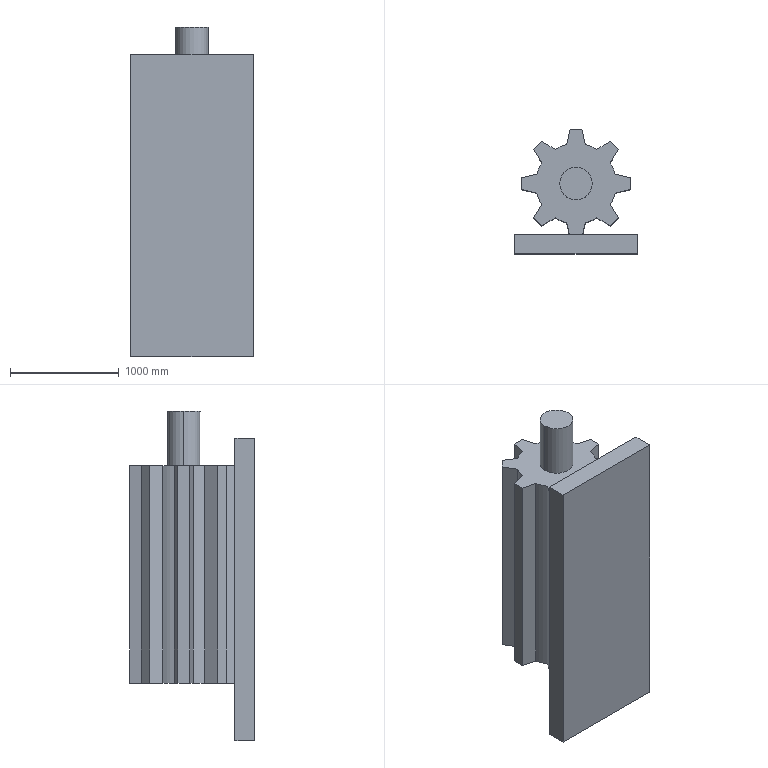Part | SolidWorks | features ICE 5, Extrusion 1 | 1 solid | 42 faces | box 1126 x 1145 x 3030 mm | volume 1733566944 mm3 | plane 32 | cylinder 10 | commonest cylinder face diameters 738.774 x8 300 x2
STEP:
#1=CARTESIAN_POINT('',(150.,0.,-3000.));
#2=VERTEX_POINT('',#1);
#3=CARTESIAN_POINT('',(-150.,0.,-3000.));
#4=VERTEX_POINT('',#3);
#5=CARTESIAN_POINT('',(0.,0.,-3000.));
#6=DIRECTION('',(0.,0.,1.));
#7=DIRECTION('',(-1.,0.,0.));
#8=AXIS2_PLACEMENT_3D('',#5,#6,#7);
#9=CIRCLE('',#8,150.);
#10=EDGE_CURVE('',#2,#4,#9,.T.);
#11=ORIENTED_EDGE('',*,*,#10,.T.);
#12=CARTESIAN_POINT('',(-150.,0.,-2500.));
#13=VERTEX_POINT('',#12);
#14=CARTESIAN_POINT('',(-150.,0.,-3000.));
#15=DIRECTION('',(0.,0.,1.));
#16=VECTOR('',#15,1000.);
#17=LINE('',#14,#16);
#18=EDGE_CURVE('',#4,#13,#17,.T.);
#19=ORIENTED_EDGE('',*,*,#18,.T.);
#20=CARTESIAN_POINT('',(150.,0.,-2500.));
#21=VERTEX_POINT('',#20);
#22=CARTESIAN_POINT('',(0.,0.,-2500.));
#23=DIRECTION('',(0.,0.,-1.));
#24=DIRECTION('',(1.,0.,0.));
#25=AXIS2_PLACEMENT_3D('',#22,#23,#24);
#26=CIRCLE('',#25,150.);
#27=EDGE_CURVE('',#13,#21,#26,.T.);
#28=ORIENTED_EDGE('',*,*,#27,.T.);
#29=CARTESIAN_POINT('',(150.,0.,-3000.));
#30=DIRECTION('',(0.,0.,1.));
#31=VECTOR('',#30,1000.);
#32=LINE('',#29,#31);
#33=EDGE_CURVE('',#2,#21,#32,.T.);
#34=ORIENTED_EDGE('',*,*,#33,.F.);
#35=EDGE_LOOP('',(#11,#19,#28,#34));
#36=FACE_OUTER_BOUND('',#35,.T.);
#37=CARTESIAN_POINT('',(0.,0.,-3000.));
#38=DIRECTION('',(0.,0.,1.));
#39=DIRECTION('',(1.,0.,0.));
#40=AXIS2_PLACEMENT_3D('',#37,#38,#39);
#41=CYLINDRICAL_SURFACE('',#40,150.);
#42=ADVANCED_FACE('',(#36),#41,.T.);
#43=ORIENTED_EDGE('',*,*,#18,.F.);
#44=CARTESIAN_POINT('',(0.,0.,-3000.));
#45=DIRECTION('',(0.,0.,1.));
#46=DIRECTION('',(-1.,0.,0.));
#47=AXIS2_PLACEMENT_3D('',#44,#45,#46);
#48=CIRCLE('',#47,150.);
#49=EDGE_CURVE('',#4,#2,#48,.T.);
#50=ORIENTED_EDGE('',*,*,#49,.T.);
#51=ORIENTED_EDGE('',*,*,#33,.T.);
#52=CARTESIAN_POINT('',(0.,0.,-2500.));
#53=DIRECTION('',(0.,0.,-1.));
#54=DIRECTION('',(1.,0.,0.));
#55=AXIS2_PLACEMENT_3D('',#52,#53,#54);
#56=CIRCLE('',#55,150.);
#57=EDGE_CURVE('',#21,#13,#56,.T.);
#58=ORIENTED_EDGE('',*,*,#57,.T.);
#59=EDGE_LOOP('',(#43,#50,#51,#58));
#60=FACE_OUTER_BOUND('',#59,.T.);
#61=CARTESIAN_POINT('',(0.,0.,-3000.));
#62=DIRECTION('',(0.,0.,1.));
#63=DIRECTION('',(1.,0.,0.));
#64=AXIS2_PLACEMENT_3D('',#61,#62,#63);
#65=CYLINDRICAL_SURFACE('',#64,150.);
#66=ADVANCED_FACE('',(#60),#65,.T.);
#67=CARTESIAN_POINT('',(60.277,-470.229,-5000.));
#68=VERTEX_POINT('',#67);
#69=CARTESIAN_POINT('',(60.277,-470.229,-3000.));
#70=VERTEX_POINT('',#69);
#71=CARTESIAN_POINT('',(60.277,-470.229,-5000.));
#72=DIRECTION('',(0.,0.,1.));
#73=VECTOR('',#72,1000.);
#74=LINE('',#71,#73);
#75=EDGE_CURVE('',#68,#70,#74,.T.);
#76=ORIENTED_EDGE('',*,*,#75,.F.);
#77=CARTESIAN_POINT('',(86.499,-359.116,-5000.));
#78=VERTEX_POINT('',#77);
#79=CARTESIAN_POINT('',(86.499,-359.116,-5000.));
#80=DIRECTION('',(-0.2297,-0.9733,0.));
#81=VECTOR('',#80,1000.);
#82=LINE('',#79,#81);
#83=EDGE_CURVE('',#78,#68,#82,.T.);
#84=ORIENTED_EDGE('',*,*,#83,.F.);
#85=CARTESIAN_POINT('',(86.499,-359.116,-3000.));
#86=VERTEX_POINT('',#85);
#87=CARTESIAN_POINT('',(86.499,-359.116,-5000.));
#88=DIRECTION('',(0.,0.,1.));
#89=VECTOR('',#88,1000.);
#90=LINE('',#87,#89);
#91=EDGE_CURVE('',#78,#86,#90,.T.);
#92=ORIENTED_EDGE('',*,*,#91,.T.);
#93=CARTESIAN_POINT('',(86.499,-359.116,-3000.));
#94=DIRECTION('',(-0.2297,-0.9733,0.));
#95=VECTOR('',#94,1000.);
#96=LINE('',#93,#95);
#97=EDGE_CURVE('',#86,#70,#96,.T.);
#98=ORIENTED_EDGE('',*,*,#97,.T.);
#99=EDGE_LOOP('',(#76,#84,#92,#98));
#100=FACE_OUTER_BOUND('',#99,.T.);
#101=CARTESIAN_POINT('',(86.499,-359.116,-5000.));
#102=DIRECTION('',(-0.9733,0.2297,0.));
#103=DIRECTION('',(-0.2297,-0.9733,0.));
#104=AXIS2_PLACEMENT_3D('',#101,#102,#103);
#105=PLANE('',#104);
#106=ADVANCED_FACE('',(#100),#105,.F.);
#107=CARTESIAN_POINT('',(-60.277,-470.229,-3000.));
#108=VERTEX_POINT('',#107);
#109=CARTESIAN_POINT('',(-60.277,-470.229,-5000.));
#110=VERTEX_POINT('',#109);
#111=CARTESIAN_POINT('',(-60.277,-470.229,-5000.));
#112=DIRECTION('',(0.,0.,-1.));
#113=VECTOR('',#112,1000.);
#114=LINE('',#111,#113);
#115=EDGE_CURVE('',#108,#110,#114,.T.);
#116=ORIENTED_EDGE('',*,*,#115,.F.);
#117=CARTESIAN_POINT('',(-86.499,-359.116,-3000.));
#118=VERTEX_POINT('',#117);
#119=CARTESIAN_POINT('',(-86.499,-359.116,-3000.));
#120=DIRECTION('',(-0.2297,0.9733,0.));
#121=VECTOR('',#120,1000.);
#122=LINE('',#119,#121);
#123=EDGE_CURVE('',#108,#118,#122,.T.);
#124=ORIENTED_EDGE('',*,*,#123,.T.);
#125=CARTESIAN_POINT('',(-86.499,-359.116,-5000.));
#126=VERTEX_POINT('',#125);
#127=CARTESIAN_POINT('',(-86.499,-359.116,-5000.));
#128=DIRECTION('',(0.,0.,1.));
#129=VECTOR('',#128,1000.);
#130=LINE('',#127,#129);
#131=EDGE_CURVE('',#126,#118,#130,.T.);
#132=ORIENTED_EDGE('',*,*,#131,.F.);
#133=CARTESIAN_POINT('',(-86.499,-359.116,-5000.));
#134=DIRECTION('',(-0.2297,0.9733,0.));
#135=VECTOR('',#134,1000.);
#136=LINE('',#133,#135);
#137=EDGE_CURVE('',#110,#126,#136,.T.);
#138=ORIENTED_EDGE('',*,*,#137,.F.);
#139=EDGE_LOOP('',(#116,#124,#132,#138));
#140=FACE_OUTER_BOUND('',#139,.T.);
#141=CARTESIAN_POINT('',(-86.499,-359.116,-5000.));
#142=DIRECTION('',(0.9733,0.2297,0.));
#143=DIRECTION('',(-0.2297,0.9733,0.));
#144=AXIS2_PLACEMENT_3D('',#141,#142,#143);
#145=PLANE('',#144);
#146=ADVANCED_FACE('',(#140),#145,.F.);
#147=ORIENTED_EDGE('',*,*,#83,.T.);
#148=CARTESIAN_POINT('',(0.,-470.229,-5000.));
#149=DIRECTION('',(-1.,0.,0.));
#150=VECTOR('',#149,1000.);
#151=LINE('',#148,#150);
#152=EDGE_CURVE('',#68,#110,#151,.T.);
#153=ORIENTED_EDGE('',*,*,#152,.T.);
#154=ORIENTED_EDGE('',*,*,#137,.T.);
#155=CARTESIAN_POINT('',(-192.769,-315.098,-5000.));
#156=VERTEX_POINT('',#155);
#157=CARTESIAN_POINT('',(0.,0.,-5000.));
#158=DIRECTION('',(0.,0.,-1.));
#159=DIRECTION('',(-1.,0.,0.));
#160=AXIS2_PLACEMENT_3D('',#157,#158,#159);
#161=CIRCLE('',#160,369.387);
#162=EDGE_CURVE('',#126,#156,#161,.T.);
#163=ORIENTED_EDGE('',*,*,#162,.T.);
#164=CARTESIAN_POINT('',(-313.695,-389.845,-5000.));
#165=VERTEX_POINT('',#164);
#166=CARTESIAN_POINT('',(-192.769,-315.098,-5000.));
#167=DIRECTION('',(-0.8506,-0.5258,0.));
#168=VECTOR('',#167,1000.);
#169=LINE('',#166,#168);
#170=EDGE_CURVE('',#156,#165,#169,.T.);
#171=ORIENTED_EDGE('',*,*,#170,.T.);
#172=CARTESIAN_POINT('',(-389.845,-313.695,-5000.));
#173=VERTEX_POINT('',#172);
#174=CARTESIAN_POINT('',(-389.845,-313.695,-5000.));
#175=DIRECTION('',(-0.7071,0.7071,0.));
#176=VECTOR('',#175,1000.);
#177=LINE('',#174,#176);
#178=EDGE_CURVE('',#165,#173,#177,.T.);
#179=ORIENTED_EDGE('',*,*,#178,.T.);
#180=CARTESIAN_POINT('',(-315.098,-192.769,-5000.));
#181=VERTEX_POINT('',#180);
#182=CARTESIAN_POINT('',(-315.098,-192.769,-5000.));
#183=DIRECTION('',(0.5258,0.8506,0.));
#184=VECTOR('',#183,1000.);
#185=LINE('',#182,#184);
#186=EDGE_CURVE('',#173,#181,#185,.T.);
#187=ORIENTED_EDGE('',*,*,#186,.T.);
#188=CARTESIAN_POINT('',(-359.116,-86.499,-5000.));
#189=VERTEX_POINT('',#188);
#190=CARTESIAN_POINT('',(0.,0.,-5000.));
#191=DIRECTION('',(0.,0.,-1.));
#192=DIRECTION('',(-1.,0.,0.));
#193=AXIS2_PLACEMENT_3D('',#190,#191,#192);
#194=CIRCLE('',#193,369.387);
#195=EDGE_CURVE('',#181,#189,#194,.T.);
#196=ORIENTED_EDGE('',*,*,#195,.T.);
#197=CARTESIAN_POINT('',(-497.478,-53.847,-5000.));
#198=VERTEX_POINT('',#197);
#199=CARTESIAN_POINT('',(-359.116,-86.499,-5000.));
#200=DIRECTION('',(-0.9733,0.2297,0.));
#201=VECTOR('',#200,1000.);
#202=LINE('',#199,#201);
#203=EDGE_CURVE('',#189,#198,#202,.T.);
#204=ORIENTED_EDGE('',*,*,#203,.T.);
#205=CARTESIAN_POINT('',(-497.478,53.847,-5000.));
#206=VERTEX_POINT('',#205);
#207=CARTESIAN_POINT('',(-497.478,53.847,-5000.));
#208=DIRECTION('',(0.,1.,0.));
#209=VECTOR('',#208,1000.);
#210=LINE('',#207,#209);
#211=EDGE_CURVE('',#198,#206,#210,.T.);
#212=ORIENTED_EDGE('',*,*,#211,.T.);
#213=CARTESIAN_POINT('',(-359.116,86.499,-5000.));
#214=VERTEX_POINT('',#213);
#215=CARTESIAN_POINT('',(-359.116,86.499,-5000.));
#216=DIRECTION('',(0.9733,0.2297,0.));
#217=VECTOR('',#216,1000.);
#218=LINE('',#215,#217);
#219=EDGE_CURVE('',#206,#214,#218,.T.);
#220=ORIENTED_EDGE('',*,*,#219,.T.);
#221=CARTESIAN_POINT('',(-315.098,192.769,-5000.));
#222=VERTEX_POINT('',#221);
#223=CARTESIAN_POINT('',(0.,0.,-5000.));
#224=DIRECTION('',(0.,0.,-1.));
#225=DIRECTION('',(-1.,0.,0.));
#226=AXIS2_PLACEMENT_3D('',#223,#224,#225);
#227=CIRCLE('',#226,369.387);
#228=EDGE_CURVE('',#214,#222,#227,.T.);
#229=ORIENTED_EDGE('',*,*,#228,.T.);
#230=CARTESIAN_POINT('',(-389.845,313.695,-5000.));
#231=VERTEX_POINT('',#230);
#232=CARTESIAN_POINT('',(-315.098,192.769,-5000.));
#233=DIRECTION('',(-0.5258,0.8506,0.));
#234=VECTOR('',#233,1000.);
#235=LINE('',#232,#234);
#236=EDGE_CURVE('',#222,#231,#235,.T.);
#237=ORIENTED_EDGE('',*,*,#236,.T.);
#238=CARTESIAN_POINT('',(-313.695,389.845,-5000.));
#239=VERTEX_POINT('',#238);
#240=CARTESIAN_POINT('',(-313.695,389.845,-5000.));
#241=DIRECTION('',(0.7071,0.7071,0.));
#242=VECTOR('',#241,1000.);
#243=LINE('',#240,#242);
#244=EDGE_CURVE('',#231,#239,#243,.T.);
#245=ORIENTED_EDGE('',*,*,#244,.T.);
#246=CARTESIAN_POINT('',(-192.769,315.098,-5000.));
#247=VERTEX_POINT('',#246);
#248=CARTESIAN_POINT('',(-192.769,315.098,-5000.));
#249=DIRECTION('',(0.8506,-0.5258,0.));
#250=VECTOR('',#249,1000.);
#251=LINE('',#248,#250);
#252=EDGE_CURVE('',#239,#247,#251,.T.);
#253=ORIENTED_EDGE('',*,*,#252,.T.);
#254=CARTESIAN_POINT('',(-86.499,359.116,-5000.));
#255=VERTEX_POINT('',#254);
#256=CARTESIAN_POINT('',(0.,0.,-5000.));
#257=DIRECTION('',(0.,0.,-1.));
#258=DIRECTION('',(-1.,0.,0.));
#259=AXIS2_PLACEMENT_3D('',#256,#257,#258);
#260=CIRCLE('',#259,369.387);
#261=EDGE_CURVE('',#247,#255,#260,.T.);
#262=ORIENTED_EDGE('',*,*,#261,.T.);
#263=CARTESIAN_POINT('',(-53.847,497.478,-5000.));
#264=VERTEX_POINT('',#263);
#265=CARTESIAN_POINT('',(-86.499,359.116,-5000.));
#266=DIRECTION('',(0.2297,0.9733,0.));
#267=VECTOR('',#266,1000.);
#268=LINE('',#265,#267);
#269=EDGE_CURVE('',#255,#264,#268,.T.);
#270=ORIENTED_EDGE('',*,*,#269,.T.);
#271=CARTESIAN_POINT('',(53.847,497.478,-5000.));
#272=VERTEX_POINT('',#271);
#273=CARTESIAN_POINT('',(53.847,497.478,-5000.));
#274=DIRECTION('',(1.,0.,0.));
#275=VECTOR('',#274,1000.);
#276=LINE('',#273,#275);
#277=EDGE_CURVE('',#264,#272,#276,.T.);
#278=ORIENTED_EDGE('',*,*,#277,.T.);
#279=CARTESIAN_POINT('',(86.499,359.116,-5000.));
#280=VERTEX_POINT('',#279);
#281=CARTESIAN_POINT('',(86.499,359.116,-5000.));
#282=DIRECTION('',(0.2297,-0.9733,0.));
#283=VECTOR('',#282,1000.);
#284=LINE('',#281,#283);
#285=EDGE_CURVE('',#272,#280,#284,.T.);
#286=ORIENTED_EDGE('',*,*,#285,.T.);
#287=CARTESIAN_POINT('',(192.769,315.098,-5000.));
#288=VERTEX_POINT('',#287);
#289=CARTESIAN_POINT('',(0.,0.,-5000.));
#290=DIRECTION('',(0.,0.,-1.));
#291=DIRECTION('',(-1.,0.,0.));
#292=AXIS2_PLACEMENT_3D('',#289,#290,#291);
#293=CIRCLE('',#292,369.387);
#294=EDGE_CURVE('',#280,#288,#293,.T.);
#295=ORIENTED_EDGE('',*,*,#294,.T.);
#296=CARTESIAN_POINT('',(313.695,389.845,-5000.));
#297=VERTEX_POINT('',#296);
#298=CARTESIAN_POINT('',(192.769,315.098,-5000.));
#299=DIRECTION('',(0.8506,0.5258,0.));
#300=VECTOR('',#299,1000.);
#301=LINE('',#298,#300);
#302=EDGE_CURVE('',#288,#297,#301,.T.);
#303=ORIENTED_EDGE('',*,*,#302,.T.);
#304=CARTESIAN_POINT('',(389.845,313.695,-5000.));
#305=VERTEX_POINT('',#304);
#306=CARTESIAN_POINT('',(389.845,313.695,-5000.));
#307=DIRECTION('',(0.7071,-0.7071,0.));
#308=VECTOR('',#307,1000.);
#309=LINE('',#306,#308);
#310=EDGE_CURVE('',#297,#305,#309,.T.);
#311=ORIENTED_EDGE('',*,*,#310,.T.);
#312=CARTESIAN_POINT('',(315.098,192.769,-5000.));
#313=VERTEX_POINT('',#312);
#314=CARTESIAN_POINT('',(315.098,192.769,-5000.));
#315=DIRECTION('',(-0.5258,-0.8506,0.));
#316=VECTOR('',#315,1000.);
#317=LINE('',#314,#316);
#318=EDGE_CURVE('',#305,#313,#317,.T.);
#319=ORIENTED_EDGE('',*,*,#318,.T.);
#320=CARTESIAN_POINT('',(359.116,86.499,-5000.));
#321=VERTEX_POINT('',#320);
#322=CARTESIAN_POINT('',(0.,0.,-5000.));
#323=DIRECTION('',(0.,0.,-1.));
#324=DIRECTION('',(-1.,0.,0.));
#325=AXIS2_PLACEMENT_3D('',#322,#323,#324);
#326=CIRCLE('',#325,369.387);
#327=EDGE_CURVE('',#313,#321,#326,.T.);
#328=ORIENTED_EDGE('',*,*,#327,.T.);
#329=CARTESIAN_POINT('',(497.478,53.847,-5000.));
#330=VERTEX_POINT('',#329);
#331=CARTESIAN_POINT('',(359.116,86.499,-5000.));
#332=DIRECTION('',(0.9733,-0.2297,0.));
#333=VECTOR('',#332,1000.);
#334=LINE('',#331,#333);
#335=EDGE_CURVE('',#321,#330,#334,.T.);
#336=ORIENTED_EDGE('',*,*,#335,.T.);
#337=CARTESIAN_POINT('',(497.478,-53.847,-5000.));
#338=VERTEX_POINT('',#337);
#339=CARTESIAN_POINT('',(497.478,-53.847,-5000.));
#340=DIRECTION('',(0.,-1.,0.));
#341=VECTOR('',#340,1000.);
#342=LINE('',#339,#341);
#343=EDGE_CURVE('',#330,#338,#342,.T.);
#344=ORIENTED_EDGE('',*,*,#343,.T.);
#345=CARTESIAN_POINT('',(359.116,-86.499,-5000.));
#346=VERTEX_POINT('',#345);
#347=CARTESIAN_POINT('',(359.116,-86.499,-5000.));
#348=DIRECTION('',(-0.9733,-0.2297,0.));
#349=VECTOR('',#348,1000.);
#350=LINE('',#347,#349);
#351=EDGE_CURVE('',#338,#346,#350,.T.);
#352=ORIENTED_EDGE('',*,*,#351,.T.);
#353=CARTESIAN_POINT('',(315.098,-192.769,-5000.));
#354=VERTEX_POINT('',#353);
#355=CARTESIAN_POINT('',(0.,0.,-5000.));
#356=DIRECTION('',(0.,0.,-1.));
#357=DIRECTION('',(-1.,0.,0.));
#358=AXIS2_PLACEMENT_3D('',#355,#356,#357);
#359=CIRCLE('',#358,369.387);
#360=EDGE_CURVE('',#346,#354,#359,.T.);
#361=ORIENTED_EDGE('',*,*,#360,.T.);
#362=CARTESIAN_POINT('',(389.845,-313.695,-5000.));
#363=VERTEX_POINT('',#362);
#364=CARTESIAN_POINT('',(315.098,-192.769,-5000.));
#365=DIRECTION('',(0.5258,-0.8506,0.));
#366=VECTOR('',#365,1000.);
#367=LINE('',#364,#366);
#368=EDGE_CURVE('',#354,#363,#367,.T.);
#369=ORIENTED_EDGE('',*,*,#368,.T.);
#370=CARTESIAN_POINT('',(313.695,-389.845,-5000.));
#371=VERTEX_POINT('',#370);
#372=CARTESIAN_POINT('',(313.695,-389.845,-5000.));
#373=DIRECTION('',(-0.7071,-0.7071,0.));
#374=VECTOR('',#373,1000.);
#375=LINE('',#372,#374);
#376=EDGE_CURVE('',#363,#371,#375,.T.);
#377=ORIENTED_EDGE('',*,*,#376,.T.);
#378=CARTESIAN_POINT('',(192.769,-315.098,-5000.));
#379=VERTEX_POINT('',#378);
#380=CARTESIAN_POINT('',(192.769,-315.098,-5000.));
#381=DIRECTION('',(-0.8506,0.5258,0.));
#382=VECTOR('',#381,1000.);
#383=LINE('',#380,#382);
#384=EDGE_CURVE('',#371,#379,#383,.T.);
#385=ORIENTED_EDGE('',*,*,#384,.T.);
#386=CARTESIAN_POINT('',(0.,0.,-5000.));
#387=DIRECTION('',(0.,0.,-1.));
#388=DIRECTION('',(-1.,0.,0.));
#389=AXIS2_PLACEMENT_3D('',#386,#387,#388);
#390=CIRCLE('',#389,369.387);
#391=EDGE_CURVE('',#379,#78,#390,.T.);
#392=ORIENTED_EDGE('',*,*,#391,.T.);
#393=EDGE_LOOP('',(#147,#153,#154,#163,#171,#179,#187,#196,#204,#212,#220,#229,#237,#245,#253,#262,#270,#278,#286,#295,#303,#311,#319,#328,#336,#344,#352,#361,#369,#377,#385,#392));
#394=FACE_OUTER_BOUND('',#393,.T.);
#395=CARTESIAN_POINT('',(0.,0.,-5000.));
#396=DIRECTION('',(0.,0.,-1.));
#397=DIRECTION('',(-1.,0.,0.));
#398=AXIS2_PLACEMENT_3D('',#395,#396,#397);
#399=PLANE('',#398);
#400=ADVANCED_FACE('',(#394),#399,.T.);
#401=ORIENTED_EDGE('',*,*,#10,.F.);
#402=ORIENTED_EDGE('',*,*,#49,.F.);
#403=EDGE_LOOP('',(#401,#402));
#404=FACE_BOUND('',#403,.T.);
#405=CARTESIAN_POINT('',(0.,-470.229,-3000.));
#406=DIRECTION('',(-1.,0.,0.));
#407=VECTOR('',#406,1000.);
#408=LINE('',#405,#407);
#409=EDGE_CURVE('',#70,#108,#408,.T.);
#410=ORIENTED_EDGE('',*,*,#409,.F.);
#411=ORIENTED_EDGE('',*,*,#97,.F.);
#412=CARTESIAN_POINT('',(192.769,-315.098,-3000.));
#413=VERTEX_POINT('',#412);
#414=CARTESIAN_POINT('',(0.,0.,-3000.));
#415=DIRECTION('',(0.,0.,-1.));
#416=DIRECTION('',(-1.,0.,0.));
#417=AXIS2_PLACEMENT_3D('',#414,#415,#416);
#418=CIRCLE('',#417,369.387);
#419=EDGE_CURVE('',#413,#86,#418,.T.);
#420=ORIENTED_EDGE('',*,*,#419,.F.);
#421=CARTESIAN_POINT('',(313.695,-389.845,-3000.));
#422=VERTEX_POINT('',#421);
#423=CARTESIAN_POINT('',(192.769,-315.098,-3000.));
#424=DIRECTION('',(-0.8506,0.5258,0.));
#425=VECTOR('',#424,1000.);
#426=LINE('',#423,#425);
#427=EDGE_CURVE('',#422,#413,#426,.T.);
#428=ORIENTED_EDGE('',*,*,#427,.F.);
#429=CARTESIAN_POINT('',(389.845,-313.695,-3000.));
#430=VERTEX_POINT('',#429);
#431=CARTESIAN_POINT('',(313.695,-389.845,-3000.));
#432=DIRECTION('',(-0.7071,-0.7071,0.));
#433=VECTOR('',#432,1000.);
#434=LINE('',#431,#433);
#435=EDGE_CURVE('',#430,#422,#434,.T.);
#436=ORIENTED_EDGE('',*,*,#435,.F.);
#437=CARTESIAN_POINT('',(315.098,-192.769,-3000.));
#438=VERTEX_POINT('',#437);
#439=CARTESIAN_POINT('',(315.098,-192.769,-3000.));
#440=DIRECTION('',(0.5258,-0.8506,0.));
#441=VECTOR('',#440,1000.);
#442=LINE('',#439,#441);
#443=EDGE_CURVE('',#438,#430,#442,.T.);
#444=ORIENTED_EDGE('',*,*,#443,.F.);
#445=CARTESIAN_POINT('',(359.116,-86.499,-3000.));
#446=VERTEX_POINT('',#445);
#447=CARTESIAN_POINT('',(0.,0.,-3000.));
#448=DIRECTION('',(0.,0.,-1.));
#449=DIRECTION('',(-1.,0.,0.));
#450=AXIS2_PLACEMENT_3D('',#447,#448,#449);
#451=CIRCLE('',#450,369.387);
#452=EDGE_CURVE('',#446,#438,#451,.T.);
#453=ORIENTED_EDGE('',*,*,#452,.F.);
#454=CARTESIAN_POINT('',(497.478,-53.847,-3000.));
#455=VERTEX_POINT('',#454);
#456=CARTESIAN_POINT('',(359.116,-86.499,-3000.));
#457=DIRECTION('',(-0.9733,-0.2297,0.));
#458=VECTOR('',#457,1000.);
#459=LINE('',#456,#458);
#460=EDGE_CURVE('',#455,#446,#459,.T.);
#461=ORIENTED_EDGE('',*,*,#460,.F.);
#462=CARTESIAN_POINT('',(497.478,53.847,-3000.));
#463=VERTEX_POINT('',#462);
#464=CARTESIAN_POINT('',(497.478,-53.847,-3000.));
#465=DIRECTION('',(0.,-1.,0.));
#466=VECTOR('',#465,1000.);
#467=LINE('',#464,#466);
#468=EDGE_CURVE('',#463,#455,#467,.T.);
#469=ORIENTED_EDGE('',*,*,#468,.F.);
#470=CARTESIAN_POINT('',(359.116,86.499,-3000.));
#471=VERTEX_POINT('',#470);
#472=CARTESIAN_POINT('',(359.116,86.499,-3000.));
#473=DIRECTION('',(0.9733,-0.2297,0.));
#474=VECTOR('',#473,1000.);
#475=LINE('',#472,#474);
#476=EDGE_CURVE('',#471,#463,#475,.T.);
#477=ORIENTED_EDGE('',*,*,#476,.F.);
#478=CARTESIAN_POINT('',(315.098,192.769,-3000.));
#479=VERTEX_POINT('',#478);
#480=CARTESIAN_POINT('',(0.,0.,-3000.));
#481=DIRECTION('',(0.,0.,-1.));
#482=DIRECTION('',(-1.,0.,0.));
#483=AXIS2_PLACEMENT_3D('',#480,#481,#482);
#484=CIRCLE('',#483,369.387);
#485=EDGE_CURVE('',#479,#471,#484,.T.);
#486=ORIENTED_EDGE('',*,*,#485,.F.);
#487=CARTESIAN_POINT('',(389.845,313.695,-3000.));
#488=VERTEX_POINT('',#487);
#489=CARTESIAN_POINT('',(315.098,192.769,-3000.));
#490=DIRECTION('',(-0.5258,-0.8506,0.));
#491=VECTOR('',#490,1000.);
#492=LINE('',#489,#491);
#493=EDGE_CURVE('',#488,#479,#492,.T.);
#494=ORIENTED_EDGE('',*,*,#493,.F.);
#495=CARTESIAN_POINT('',(313.695,389.845,-3000.));
#496=VERTEX_POINT('',#495);
#497=CARTESIAN_POINT('',(389.845,313.695,-3000.));
#498=DIRECTION('',(0.7071,-0.7071,0.));
#499=VECTOR('',#498,1000.);
#500=LINE('',#497,#499);
#501=EDGE_CURVE('',#496,#488,#500,.T.);
#502=ORIENTED_EDGE('',*,*,#501,.F.);
#503=CARTESIAN_POINT('',(192.769,315.098,-3000.));
#504=VERTEX_POINT('',#503);
#505=CARTESIAN_POINT('',(192.769,315.098,-3000.));
#506=DIRECTION('',(0.8506,0.5258,0.));
#507=VECTOR('',#506,1000.);
#508=LINE('',#505,#507);
#509=EDGE_CURVE('',#504,#496,#508,.T.);
#510=ORIENTED_EDGE('',*,*,#509,.F.);
#511=CARTESIAN_POINT('',(86.499,359.116,-3000.));
#512=VERTEX_POINT('',#511);
#513=CARTESIAN_POINT('',(0.,0.,-3000.));
#514=DIRECTION('',(0.,0.,-1.));
#515=DIRECTION('',(-1.,0.,0.));
#516=AXIS2_PLACEMENT_3D('',#513,#514,#515);
#517=CIRCLE('',#516,369.387);
#518=EDGE_CURVE('',#512,#504,#517,.T.);
#519=ORIENTED_EDGE('',*,*,#518,.F.);
#520=CARTESIAN_POINT('',(53.847,497.478,-3000.));
#521=VERTEX_POINT('',#520);
#522=CARTESIAN_POINT('',(86.499,359.116,-3000.));
#523=DIRECTION('',(0.2297,-0.9733,0.));
#524=VECTOR('',#523,1000.);
#525=LINE('',#522,#524);
#526=EDGE_CURVE('',#521,#512,#525,.T.);
#527=ORIENTED_EDGE('',*,*,#526,.F.);
#528=CARTESIAN_POINT('',(-53.847,497.478,-3000.));
#529=VERTEX_POINT('',#528);
#530=CARTESIAN_POINT('',(53.847,497.478,-3000.));
#531=DIRECTION('',(1.,0.,0.));
#532=VECTOR('',#531,1000.);
#533=LINE('',#530,#532);
#534=EDGE_CURVE('',#529,#521,#533,.T.);
#535=ORIENTED_EDGE('',*,*,#534,.F.);
#536=CARTESIAN_POINT('',(-86.499,359.116,-3000.));
#537=VERTEX_POINT('',#536);
#538=CARTESIAN_POINT('',(-86.499,359.116,-3000.));
#539=DIRECTION('',(0.2297,0.9733,0.));
#540=VECTOR('',#539,1000.);
#541=LINE('',#538,#540);
#542=EDGE_CURVE('',#537,#529,#541,.T.);
#543=ORIENTED_EDGE('',*,*,#542,.F.);
#544=CARTESIAN_POINT('',(-192.769,315.098,-3000.));
#545=VERTEX_POINT('',#544);
#546=CARTESIAN_POINT('',(0.,0.,-3000.));
#547=DIRECTION('',(0.,0.,-1.));
#548=DIRECTION('',(-1.,0.,0.));
#549=AXIS2_PLACEMENT_3D('',#546,#547,#548);
#550=CIRCLE('',#549,369.387);
#551=EDGE_CURVE('',#545,#537,#550,.T.);
#552=ORIENTED_EDGE('',*,*,#551,.F.);
#553=CARTESIAN_POINT('',(-313.695,389.845,-3000.));
#554=VERTEX_POINT('',#553);
#555=CARTESIAN_POINT('',(-192.769,315.098,-3000.));
#556=DIRECTION('',(0.8506,-0.5258,0.));
#557=VECTOR('',#556,1000.);
#558=LINE('',#555,#557);
#559=EDGE_CURVE('',#554,#545,#558,.T.);
#560=ORIENTED_EDGE('',*,*,#559,.F.);
#561=CARTESIAN_POINT('',(-389.845,313.695,-3000.));
#562=VERTEX_POINT('',#561);
#563=CARTESIAN_POINT('',(-313.695,389.845,-3000.));
#564=DIRECTION('',(0.7071,0.7071,0.));
#565=VECTOR('',#564,1000.);
#566=LINE('',#563,#565);
#567=EDGE_CURVE('',#562,#554,#566,.T.);
#568=ORIENTED_EDGE('',*,*,#567,.F.);
#569=CARTESIAN_POINT('',(-315.098,192.769,-3000.));
#570=VERTEX_POINT('',#569);
#571=CARTESIAN_POINT('',(-315.098,192.769,-3000.));
#572=DIRECTION('',(-0.5258,0.8506,0.));
#573=VECTOR('',#572,1000.);
#574=LINE('',#571,#573);
#575=EDGE_CURVE('',#570,#562,#574,.T.);
#576=ORIENTED_EDGE('',*,*,#575,.F.);
#577=CARTESIAN_POINT('',(-359.116,86.499,-3000.));
#578=VERTEX_POINT('',#577);
#579=CARTESIAN_POINT('',(0.,0.,-3000.));
#580=DIRECTION('',(0.,0.,-1.));
#581=DIRECTION('',(-1.,0.,0.));
#582=AXIS2_PLACEMENT_3D('',#579,#580,#581);
#583=CIRCLE('',#582,369.387);
#584=EDGE_CURVE('',#578,#570,#583,.T.);
#585=ORIENTED_EDGE('',*,*,#584,.F.);
#586=CARTESIAN_POINT('',(-497.478,53.847,-3000.));
#587=VERTEX_POINT('',#586);
#588=CARTESIAN_POINT('',(-359.116,86.499,-3000.));
#589=DIRECTION('',(0.9733,0.2297,0.));
#590=VECTOR('',#589,1000.);
#591=LINE('',#588,#590);
#592=EDGE_CURVE('',#587,#578,#591,.T.);
#593=ORIENTED_EDGE('',*,*,#592,.F.);
#594=CARTESIAN_POINT('',(-497.478,-53.847,-3000.));
#595=VERTEX_POINT('',#594);
#596=CARTESIAN_POINT('',(-497.478,53.847,-3000.));
#597=DIRECTION('',(0.,1.,0.));
#598=VECTOR('',#597,1000.);
#599=LINE('',#596,#598);
#600=EDGE_CURVE('',#595,#587,#599,.T.);
#601=ORIENTED_EDGE('',*,*,#600,.F.);
#602=CARTESIAN_POINT('',(-359.116,-86.499,-3000.));
#603=VERTEX_POINT('',#602);
#604=CARTESIAN_POINT('',(-359.116,-86.499,-3000.));
#605=DIRECTION('',(-0.9733,0.2297,0.));
#606=VECTOR('',#605,1000.);
#607=LINE('',#604,#606);
#608=EDGE_CURVE('',#603,#595,#607,.T.);
#609=ORIENTED_EDGE('',*,*,#608,.F.);
#610=CARTESIAN_POINT('',(-315.098,-192.769,-3000.));
#611=VERTEX_POINT('',#610);
#612=CARTESIAN_POINT('',(0.,0.,-3000.));
#613=DIRECTION('',(0.,0.,-1.));
#614=DIRECTION('',(-1.,0.,0.));
#615=AXIS2_PLACEMENT_3D('',#612,#613,#614);
#616=CIRCLE('',#615,369.387);
#617=EDGE_CURVE('',#611,#603,#616,.T.);
#618=ORIENTED_EDGE('',*,*,#617,.F.);
#619=CARTESIAN_POINT('',(-389.845,-313.695,-3000.));
#620=VERTEX_POINT('',#619);
#621=CARTESIAN_POINT('',(-315.098,-192.769,-3000.));
#622=DIRECTION('',(0.5258,0.8506,0.));
#623=VECTOR('',#622,1000.);
#624=LINE('',#621,#623);
#625=EDGE_CURVE('',#620,#611,#624,.T.);
#626=ORIENTED_EDGE('',*,*,#625,.F.);
#627=CARTESIAN_POINT('',(-313.695,-389.845,-3000.));
#628=VERTEX_POINT('',#627);
#629=CARTESIAN_POINT('',(-389.845,-313.695,-3000.));
#630=DIRECTION('',(-0.7071,0.7071,0.));
#631=VECTOR('',#630,1000.);
#632=LINE('',#629,#631);
#633=EDGE_CURVE('',#628,#620,#632,.T.);
#634=ORIENTED_EDGE('',*,*,#633,.F.);
#635=CARTESIAN_POINT('',(-192.769,-315.098,-3000.));
#636=VERTEX_POINT('',#635);
#637=CARTESIAN_POINT('',(-192.769,-315.098,-3000.));
#638=DIRECTION('',(-0.8506,-0.5258,0.));
#639=VECTOR('',#638,1000.);
#640=LINE('',#637,#639);
#641=EDGE_CURVE('',#636,#628,#640,.T.);
#642=ORIENTED_EDGE('',*,*,#641,.F.);
#643=CARTESIAN_POINT('',(0.,0.,-3000.));
#644=DIRECTION('',(0.,0.,-1.));
#645=DIRECTION('',(-1.,0.,0.));
#646=AXIS2_PLACEMENT_3D('',#643,#644,#645);
#647=CIRCLE('',#646,369.387);
#648=EDGE_CURVE('',#118,#636,#647,.T.);
#649=ORIENTED_EDGE('',*,*,#648,.F.);
#650=ORIENTED_EDGE('',*,*,#123,.F.);
#651=EDGE_LOOP('',(#410,#411,#420,#428,#436,#444,#453,#461,#469,#477,#486,#494,#502,#510,#519,#527,#535,#543,#552,#560,#568,#576,#585,#593,#601,#609,#618,#626,#634,#642,#649,#650));
#652=FACE_OUTER_BOUND('',#651,.T.);
#653=CARTESIAN_POINT('',(0.,0.,-3000.));
#654=DIRECTION('',(0.,0.,-1.));
#655=DIRECTION('',(-1.,0.,0.));
#656=AXIS2_PLACEMENT_3D('',#653,#654,#655);
#657=PLANE('',#656);
#658=ADVANCED_FACE('',(#404,#652),#657,.F.);
#659=ORIENTED_EDGE('',*,*,#518,.T.);
#660=CARTESIAN_POINT('',(192.769,315.098,-5000.));
#661=DIRECTION('',(0.,0.,1.));
#662=VECTOR('',#661,1000.);
#663=LINE('',#660,#662);
#664=EDGE_CURVE('',#288,#504,#663,.T.);
#665=ORIENTED_EDGE('',*,*,#664,.F.);
#666=ORIENTED_EDGE('',*,*,#294,.F.);
#667=CARTESIAN_POINT('',(86.499,359.116,-5000.));
#668=DIRECTION('',(0.,0.,1.));
#669=VECTOR('',#668,1000.);
#670=LINE('',#667,#669);
#671=EDGE_CURVE('',#280,#512,#670,.T.);
#672=ORIENTED_EDGE('',*,*,#671,.T.);
#673=EDGE_LOOP('',(#659,#665,#666,#672));
#674=FACE_OUTER_BOUND('',#673,.T.);
#675=CARTESIAN_POINT('',(0.,0.,-5000.));
#676=DIRECTION('',(0.,0.,1.));
#677=DIRECTION('',(1.,0.,0.));
#678=AXIS2_PLACEMENT_3D('',#675,#676,#677);
#679=CYLINDRICAL_SURFACE('',#678,369.387);
#680=ADVANCED_FACE('',(#674),#679,.T.);
#681=ORIENTED_EDGE('',*,*,#509,.T.);
#682=CARTESIAN_POINT('',(313.695,389.845,-5000.));
#683=DIRECTION('',(0.,0.,1.));
#684=VECTOR('',#683,1000.);
#685=LINE('',#682,#684);
#686=EDGE_CURVE('',#297,#496,#685,.T.);
#687=ORIENTED_EDGE('',*,*,#686,.F.);
#688=ORIENTED_EDGE('',*,*,#302,.F.);
#689=ORIENTED_EDGE('',*,*,#664,.T.);
#690=EDGE_LOOP('',(#681,#687,#688,#689));
#691=FACE_OUTER_BOUND('',#690,.T.);
#692=CARTESIAN_POINT('',(192.769,315.098,-5000.));
#693=DIRECTION('',(0.5258,-0.8506,0.));
#694=DIRECTION('',(0.8506,0.5258,0.));
#695=AXIS2_PLACEMENT_3D('',#692,#693,#694);
#696=PLANE('',#695);
#697=ADVANCED_FACE('',(#691),#696,.F.);
#698=ORIENTED_EDGE('',*,*,#501,.T.);
#699=CARTESIAN_POINT('',(389.845,313.695,-5000.));
#700=DIRECTION('',(0.,0.,1.));
#701=VECTOR('',#700,1000.);
#702=LINE('',#699,#701);
#703=EDGE_CURVE('',#305,#488,#702,.T.);
#704=ORIENTED_EDGE('',*,*,#703,.F.);
#705=ORIENTED_EDGE('',*,*,#310,.F.);
#706=ORIENTED_EDGE('',*,*,#686,.T.);
#707=EDGE_LOOP('',(#698,#704,#705,#706));
#708=FACE_OUTER_BOUND('',#707,.T.);
#709=CARTESIAN_POINT('',(389.845,313.695,-5000.));
#710=DIRECTION('',(-0.7071,-0.7071,0.));
#711=DIRECTION('',(0.7071,-0.7071,0.));
#712=AXIS2_PLACEMENT_3D('',#709,#710,#711);
#713=PLANE('',#712);
#714=ADVANCED_FACE('',(#708),#713,.F.);
#715=ORIENTED_EDGE('',*,*,#493,.T.);
#716=CARTESIAN_POINT('',(315.098,192.769,-5000.));
#717=DIRECTION('',(0.,0.,1.));
#718=VECTOR('',#717,1000.);
#719=LINE('',#716,#718);
#720=EDGE_CURVE('',#313,#479,#719,.T.);
#721=ORIENTED_EDGE('',*,*,#720,.F.);
#722=ORIENTED_EDGE('',*,*,#318,.F.);
#723=ORIENTED_EDGE('',*,*,#703,.T.);
#724=EDGE_LOOP('',(#715,#721,#722,#723));
#725=FACE_OUTER_BOUND('',#724,.T.);
#726=CARTESIAN_POINT('',(315.098,192.769,-5000.));
#727=DIRECTION('',(-0.8506,0.5258,0.));
#728=DIRECTION('',(-0.5258,-0.8506,0.));
#729=AXIS2_PLACEMENT_3D('',#726,#727,#728);
#730=PLANE('',#729);
#731=ADVANCED_FACE('',(#725),#730,.F.);
#732=ORIENTED_EDGE('',*,*,#485,.T.);
#733=CARTESIAN_POINT('',(359.116,86.499,-5000.));
#734=DIRECTION('',(0.,0.,1.));
#735=VECTOR('',#734,1000.);
#736=LINE('',#733,#735);
#737=EDGE_CURVE('',#321,#471,#736,.T.);
#738=ORIENTED_EDGE('',*,*,#737,.F.);
#739=ORIENTED_EDGE('',*,*,#327,.F.);
#740=ORIENTED_EDGE('',*,*,#720,.T.);
#741=EDGE_LOOP('',(#732,#738,#739,#740));
#742=FACE_OUTER_BOUND('',#741,.T.);
#743=CARTESIAN_POINT('',(0.,0.,-5000.));
#744=DIRECTION('',(0.,0.,1.));
#745=DIRECTION('',(1.,0.,0.));
#746=AXIS2_PLACEMENT_3D('',#743,#744,#745);
#747=CYLINDRICAL_SURFACE('',#746,369.387);
#748=ADVANCED_FACE('',(#742),#747,.T.);
#749=ORIENTED_EDGE('',*,*,#476,.T.);
#750=CARTESIAN_POINT('',(497.478,53.847,-5000.));
#751=DIRECTION('',(0.,0.,1.));
#752=VECTOR('',#751,1000.);
#753=LINE('',#750,#752);
#754=EDGE_CURVE('',#330,#463,#753,.T.);
#755=ORIENTED_EDGE('',*,*,#754,.F.);
#756=ORIENTED_EDGE('',*,*,#335,.F.);
#757=ORIENTED_EDGE('',*,*,#737,.T.);
#758=EDGE_LOOP('',(#749,#755,#756,#757));
#759=FACE_OUTER_BOUND('',#758,.T.);
#760=CARTESIAN_POINT('',(359.116,86.499,-5000.));
#761=DIRECTION('',(-0.2297,-0.9733,0.));
#762=DIRECTION('',(0.9733,-0.2297,0.));
#763=AXIS2_PLACEMENT_3D('',#760,#761,#762);
#764=PLANE('',#763);
#765=ADVANCED_FACE('',(#759),#764,.F.);
#766=ORIENTED_EDGE('',*,*,#468,.T.);
#767=CARTESIAN_POINT('',(497.478,-53.847,-5000.));
#768=DIRECTION('',(0.,0.,1.));
#769=VECTOR('',#768,1000.);
#770=LINE('',#767,#769);
#771=EDGE_CURVE('',#338,#455,#770,.T.);
#772=ORIENTED_EDGE('',*,*,#771,.F.);
#773=ORIENTED_EDGE('',*,*,#343,.F.);
#774=ORIENTED_EDGE('',*,*,#754,.T.);
#775=EDGE_LOOP('',(#766,#772,#773,#774));
#776=FACE_OUTER_BOUND('',#775,.T.);
#777=CARTESIAN_POINT('',(497.478,-53.847,-5000.));
#778=DIRECTION('',(-1.,0.,0.));
#779=DIRECTION('',(0.,0.,1.));
#780=AXIS2_PLACEMENT_3D('',#777,#778,#779);
#781=PLANE('',#780);
#782=ADVANCED_FACE('',(#776),#781,.F.);
#783=ORIENTED_EDGE('',*,*,#460,.T.);
#784=CARTESIAN_POINT('',(359.116,-86.499,-5000.));
#785=DIRECTION('',(0.,0.,1.));
#786=VECTOR('',#785,1000.);
#787=LINE('',#784,#786);
#788=EDGE_CURVE('',#346,#446,#787,.T.);
#789=ORIENTED_EDGE('',*,*,#788,.F.);
#790=ORIENTED_EDGE('',*,*,#351,.F.);
#791=ORIENTED_EDGE('',*,*,#771,.T.);
#792=EDGE_LOOP('',(#783,#789,#790,#791));
#793=FACE_OUTER_BOUND('',#792,.T.);
#794=CARTESIAN_POINT('',(359.116,-86.499,-5000.));
#795=DIRECTION('',(-0.2297,0.9733,0.));
#796=DIRECTION('',(-0.9733,-0.2297,0.));
#797=AXIS2_PLACEMENT_3D('',#794,#795,#796);
#798=PLANE('',#797);
#799=ADVANCED_FACE('',(#793),#798,.F.);
#800=ORIENTED_EDGE('',*,*,#452,.T.);
#801=CARTESIAN_POINT('',(315.098,-192.769,-5000.));
#802=DIRECTION('',(0.,0.,1.));
#803=VECTOR('',#802,1000.);
#804=LINE('',#801,#803);
#805=EDGE_CURVE('',#354,#438,#804,.T.);
#806=ORIENTED_EDGE('',*,*,#805,.F.);
#807=ORIENTED_EDGE('',*,*,#360,.F.);
#808=ORIENTED_EDGE('',*,*,#788,.T.);
#809=EDGE_LOOP('',(#800,#806,#807,#808));
#810=FACE_OUTER_BOUND('',#809,.T.);
#811=CARTESIAN_POINT('',(0.,0.,-5000.));
#812=DIRECTION('',(0.,0.,1.));
#813=DIRECTION('',(1.,0.,0.));
#814=AXIS2_PLACEMENT_3D('',#811,#812,#813);
#815=CYLINDRICAL_SURFACE('',#814,369.387);
#816=ADVANCED_FACE('',(#810),#815,.T.);
#817=ORIENTED_EDGE('',*,*,#443,.T.);
#818=CARTESIAN_POINT('',(389.845,-313.695,-5000.));
#819=DIRECTION('',(0.,0.,1.));
#820=VECTOR('',#819,1000.);
#821=LINE('',#818,#820);
#822=EDGE_CURVE('',#363,#430,#821,.T.);
#823=ORIENTED_EDGE('',*,*,#822,.F.);
#824=ORIENTED_EDGE('',*,*,#368,.F.);
#825=ORIENTED_EDGE('',*,*,#805,.T.);
#826=EDGE_LOOP('',(#817,#823,#824,#825));
#827=FACE_OUTER_BOUND('',#826,.T.);
#828=CARTESIAN_POINT('',(315.098,-192.769,-5000.));
#829=DIRECTION('',(-0.8506,-0.5258,0.));
#830=DIRECTION('',(0.5258,-0.8506,0.));
#831=AXIS2_PLACEMENT_3D('',#828,#829,#830);
#832=PLANE('',#831);
#833=ADVANCED_FACE('',(#827),#832,.F.);
#834=ORIENTED_EDGE('',*,*,#435,.T.);
#835=CARTESIAN_POINT('',(313.695,-389.845,-5000.));
#836=DIRECTION('',(0.,0.,1.));
#837=VECTOR('',#836,1000.);
#838=LINE('',#835,#837);
#839=EDGE_CURVE('',#371,#422,#838,.T.);
#840=ORIENTED_EDGE('',*,*,#839,.F.);
#841=ORIENTED_EDGE('',*,*,#376,.F.);
#842=ORIENTED_EDGE('',*,*,#822,.T.);
#843=EDGE_LOOP('',(#834,#840,#841,#842));
#844=FACE_OUTER_BOUND('',#843,.T.);
#845=CARTESIAN_POINT('',(313.695,-389.845,-5000.));
#846=DIRECTION('',(-0.7071,0.7071,0.));
#847=DIRECTION('',(-0.7071,-0.7071,0.));
#848=AXIS2_PLACEMENT_3D('',#845,#846,#847);
#849=PLANE('',#848);
#850=ADVANCED_FACE('',(#844),#849,.F.);
#851=ORIENTED_EDGE('',*,*,#427,.T.);
#852=CARTESIAN_POINT('',(192.769,-315.098,-5000.));
#853=DIRECTION('',(0.,0.,1.));
#854=VECTOR('',#853,1000.);
#855=LINE('',#852,#854);
#856=EDGE_CURVE('',#379,#413,#855,.T.);
#857=ORIENTED_EDGE('',*,*,#856,.F.);
#858=ORIENTED_EDGE('',*,*,#384,.F.);
#859=ORIENTED_EDGE('',*,*,#839,.T.);
#860=EDGE_LOOP('',(#851,#857,#858,#859));
#861=FACE_OUTER_BOUND('',#860,.T.);
#862=CARTESIAN_POINT('',(192.769,-315.098,-5000.));
#863=DIRECTION('',(0.5258,0.8506,0.));
#864=DIRECTION('',(-0.8506,0.5258,0.));
#865=AXIS2_PLACEMENT_3D('',#862,#863,#864);
#866=PLANE('',#865);
#867=ADVANCED_FACE('',(#861),#866,.F.);
#868=ORIENTED_EDGE('',*,*,#419,.T.);
#869=ORIENTED_EDGE('',*,*,#91,.F.);
#870=ORIENTED_EDGE('',*,*,#391,.F.);
#871=ORIENTED_EDGE('',*,*,#856,.T.);
#872=EDGE_LOOP('',(#868,#869,#870,#871));
#873=FACE_OUTER_BOUND('',#872,.T.);
#874=CARTESIAN_POINT('',(0.,0.,-5000.));
#875=DIRECTION('',(0.,0.,1.));
#876=DIRECTION('',(1.,0.,0.));
#877=AXIS2_PLACEMENT_3D('',#874,#875,#876);
#878=CYLINDRICAL_SURFACE('',#877,369.387);
#879=ADVANCED_FACE('',(#873),#878,.T.);
#880=ORIENTED_EDGE('',*,*,#648,.T.);
#881=CARTESIAN_POINT('',(-192.769,-315.098,-5000.));
#882=DIRECTION('',(0.,0.,1.));
#883=VECTOR('',#882,1000.);
#884=LINE('',#881,#883);
#885=EDGE_CURVE('',#156,#636,#884,.T.);
#886=ORIENTED_EDGE('',*,*,#885,.F.);
#887=ORIENTED_EDGE('',*,*,#162,.F.);
#888=ORIENTED_EDGE('',*,*,#131,.T.);
#889=EDGE_LOOP('',(#880,#886,#887,#888));
#890=FACE_OUTER_BOUND('',#889,.T.);
#891=CARTESIAN_POINT('',(0.,0.,-5000.));
#892=DIRECTION('',(0.,0.,1.));
#893=DIRECTION('',(1.,0.,0.));
#894=AXIS2_PLACEMENT_3D('',#891,#892,#893);
#895=CYLINDRICAL_SURFACE('',#894,369.387);
#896=ADVANCED_FACE('',(#890),#895,.T.);
#897=ORIENTED_EDGE('',*,*,#641,.T.);
#898=CARTESIAN_POINT('',(-313.695,-389.845,-5000.));
#899=DIRECTION('',(0.,0.,1.));
#900=VECTOR('',#899,1000.);
#901=LINE('',#898,#900);
#902=EDGE_CURVE('',#165,#628,#901,.T.);
#903=ORIENTED_EDGE('',*,*,#902,.F.);
#904=ORIENTED_EDGE('',*,*,#170,.F.);
#905=ORIENTED_EDGE('',*,*,#885,.T.);
#906=EDGE_LOOP('',(#897,#903,#904,#905));
#907=FACE_OUTER_BOUND('',#906,.T.);
#908=CARTESIAN_POINT('',(-192.769,-315.098,-5000.));
#909=DIRECTION('',(-0.5258,0.8506,0.));
#910=DIRECTION('',(-0.8506,-0.5258,0.));
#911=AXIS2_PLACEMENT_3D('',#908,#909,#910);
#912=PLANE('',#911);
#913=ADVANCED_FACE('',(#907),#912,.F.);
#914=ORIENTED_EDGE('',*,*,#633,.T.);
#915=CARTESIAN_POINT('',(-389.845,-313.695,-5000.));
#916=DIRECTION('',(0.,0.,1.));
#917=VECTOR('',#916,1000.);
#918=LINE('',#915,#917);
#919=EDGE_CURVE('',#173,#620,#918,.T.);
#920=ORIENTED_EDGE('',*,*,#919,.F.);
#921=ORIENTED_EDGE('',*,*,#178,.F.);
#922=ORIENTED_EDGE('',*,*,#902,.T.);
#923=EDGE_LOOP('',(#914,#920,#921,#922));
#924=FACE_OUTER_BOUND('',#923,.T.);
#925=CARTESIAN_POINT('',(-389.845,-313.695,-5000.));
#926=DIRECTION('',(0.7071,0.7071,0.));
#927=DIRECTION('',(-0.7071,0.7071,0.));
#928=AXIS2_PLACEMENT_3D('',#925,#926,#927);
#929=PLANE('',#928);
#930=ADVANCED_FACE('',(#924),#929,.F.);
#931=ORIENTED_EDGE('',*,*,#625,.T.);
#932=CARTESIAN_POINT('',(-315.098,-192.769,-5000.));
#933=DIRECTION('',(0.,0.,1.));
#934=VECTOR('',#933,1000.);
#935=LINE('',#932,#934);
#936=EDGE_CURVE('',#181,#611,#935,.T.);
#937=ORIENTED_EDGE('',*,*,#936,.F.);
#938=ORIENTED_EDGE('',*,*,#186,.F.);
#939=ORIENTED_EDGE('',*,*,#919,.T.);
#940=EDGE_LOOP('',(#931,#937,#938,#939));
#941=FACE_OUTER_BOUND('',#940,.T.);
#942=CARTESIAN_POINT('',(-315.098,-192.769,-5000.));
#943=DIRECTION('',(0.8506,-0.5258,0.));
#944=DIRECTION('',(0.5258,0.8506,0.));
#945=AXIS2_PLACEMENT_3D('',#942,#943,#944);
#946=PLANE('',#945);
#947=ADVANCED_FACE('',(#941),#946,.F.);
#948=ORIENTED_EDGE('',*,*,#617,.T.);
#949=CARTESIAN_POINT('',(-359.116,-86.499,-5000.));
#950=DIRECTION('',(0.,0.,1.));
#951=VECTOR('',#950,1000.);
#952=LINE('',#949,#951);
#953=EDGE_CURVE('',#189,#603,#952,.T.);
#954=ORIENTED_EDGE('',*,*,#953,.F.);
#955=ORIENTED_EDGE('',*,*,#195,.F.);
#956=ORIENTED_EDGE('',*,*,#936,.T.);
#957=EDGE_LOOP('',(#948,#954,#955,#956));
#958=FACE_OUTER_BOUND('',#957,.T.);
#959=CARTESIAN_POINT('',(0.,0.,-5000.));
#960=DIRECTION('',(0.,0.,1.));
#961=DIRECTION('',(1.,0.,0.));
#962=AXIS2_PLACEMENT_3D('',#959,#960,#961);
#963=CYLINDRICAL_SURFACE('',#962,369.387);
#964=ADVANCED_FACE('',(#958),#963,.T.);
#965=ORIENTED_EDGE('',*,*,#608,.T.);
#966=CARTESIAN_POINT('',(-497.478,-53.847,-5000.));
#967=DIRECTION('',(0.,0.,1.));
#968=VECTOR('',#967,1000.);
#969=LINE('',#966,#968);
#970=EDGE_CURVE('',#198,#595,#969,.T.);
#971=ORIENTED_EDGE('',*,*,#970,.F.);
#972=ORIENTED_EDGE('',*,*,#203,.F.);
#973=ORIENTED_EDGE('',*,*,#953,.T.);
#974=EDGE_LOOP('',(#965,#971,#972,#973));
#975=FACE_OUTER_BOUND('',#974,.T.);
#976=CARTESIAN_POINT('',(-359.116,-86.499,-5000.));
#977=DIRECTION('',(0.2297,0.9733,0.));
#978=DIRECTION('',(-0.9733,0.2297,0.));
#979=AXIS2_PLACEMENT_3D('',#976,#977,#978);
#980=PLANE('',#979);
#981=ADVANCED_FACE('',(#975),#980,.F.);
#982=ORIENTED_EDGE('',*,*,#600,.T.);
#983=CARTESIAN_POINT('',(-497.478,53.847,-5000.));
#984=DIRECTION('',(0.,0.,1.));
#985=VECTOR('',#984,1000.);
#986=LINE('',#983,#985);
#987=EDGE_CURVE('',#206,#587,#986,.T.);
#988=ORIENTED_EDGE('',*,*,#987,.F.);
#989=ORIENTED_EDGE('',*,*,#211,.F.);
#990=ORIENTED_EDGE('',*,*,#970,.T.);
#991=EDGE_LOOP('',(#982,#988,#989,#990));
#992=FACE_OUTER_BOUND('',#991,.T.);
#993=CARTESIAN_POINT('',(-497.478,53.847,-5000.));
#994=DIRECTION('',(1.,0.,0.));
#995=DIRECTION('',(0.,1.,0.));
#996=AXIS2_PLACEMENT_3D('',#993,#994,#995);
#997=PLANE('',#996);
#998=ADVANCED_FACE('',(#992),#997,.F.);
#999=ORIENTED_EDGE('',*,*,#592,.T.);
#1000=CARTESIAN_POINT('',(-359.116,86.499,-5000.));
#1001=DIRECTION('',(0.,0.,1.));
#1002=VECTOR('',#1001,1000.);
#1003=LINE('',#1000,#1002);
#1004=EDGE_CURVE('',#214,#578,#1003,.T.);
#1005=ORIENTED_EDGE('',*,*,#1004,.F.);
#1006=ORIENTED_EDGE('',*,*,#219,.F.);
#1007=ORIENTED_EDGE('',*,*,#987,.T.);
#1008=EDGE_LOOP('',(#999,#1005,#1006,#1007));
#1009=FACE_OUTER_BOUND('',#1008,.T.);
#1010=CARTESIAN_POINT('',(-359.116,86.499,-5000.));
#1011=DIRECTION('',(0.2297,-0.9733,0.));
#1012=DIRECTION('',(0.9733,0.2297,0.));
#1013=AXIS2_PLACEMENT_3D('',#1010,#1011,#1012);
#1014=PLANE('',#1013);
#1015=ADVANCED_FACE('',(#1009),#1014,.F.);
#1016=ORIENTED_EDGE('',*,*,#584,.T.);
#1017=CARTESIAN_POINT('',(-315.098,192.769,-5000.));
#1018=DIRECTION('',(0.,0.,1.));
#1019=VECTOR('',#1018,1000.);
#1020=LINE('',#1017,#1019);
#1021=EDGE_CURVE('',#222,#570,#1020,.T.);
#1022=ORIENTED_EDGE('',*,*,#1021,.F.);
#1023=ORIENTED_EDGE('',*,*,#228,.F.);
#1024=ORIENTED_EDGE('',*,*,#1004,.T.);
#1025=EDGE_LOOP('',(#1016,#1022,#1023,#1024));
#1026=FACE_OUTER_BOUND('',#1025,.T.);
#1027=CARTESIAN_POINT('',(0.,0.,-5000.));
#1028=DIRECTION('',(0.,0.,1.));
#1029=DIRECTION('',(1.,0.,0.));
#1030=AXIS2_PLACEMENT_3D('',#1027,#1028,#1029);
#1031=CYLINDRICAL_SURFACE('',#1030,369.387);
#1032=ADVANCED_FACE('',(#1026),#1031,.T.);
#1033=ORIENTED_EDGE('',*,*,#575,.T.);
#1034=CARTESIAN_POINT('',(-389.845,313.695,-5000.));
#1035=DIRECTION('',(0.,0.,1.));
#1036=VECTOR('',#1035,1000.);
#1037=LINE('',#1034,#1036);
#1038=EDGE_CURVE('',#231,#562,#1037,.T.);
#1039=ORIENTED_EDGE('',*,*,#1038,.F.);
#1040=ORIENTED_EDGE('',*,*,#236,.F.);
#1041=ORIENTED_EDGE('',*,*,#1021,.T.);
#1042=EDGE_LOOP('',(#1033,#1039,#1040,#1041));
#1043=FACE_OUTER_BOUND('',#1042,.T.);
#1044=CARTESIAN_POINT('',(-315.098,192.769,-5000.));
#1045=DIRECTION('',(0.8506,0.5258,0.));
#1046=DIRECTION('',(-0.5258,0.8506,0.));
#1047=AXIS2_PLACEMENT_3D('',#1044,#1045,#1046);
#1048=PLANE('',#1047);
#1049=ADVANCED_FACE('',(#1043),#1048,.F.);
#1050=ORIENTED_EDGE('',*,*,#567,.T.);
#1051=CARTESIAN_POINT('',(-313.695,389.845,-5000.));
#1052=DIRECTION('',(0.,0.,1.));
#1053=VECTOR('',#1052,1000.);
#1054=LINE('',#1051,#1053);
#1055=EDGE_CURVE('',#239,#554,#1054,.T.);
#1056=ORIENTED_EDGE('',*,*,#1055,.F.);
#1057=ORIENTED_EDGE('',*,*,#244,.F.);
#1058=ORIENTED_EDGE('',*,*,#1038,.T.);
#1059=EDGE_LOOP('',(#1050,#1056,#1057,#1058));
#1060=FACE_OUTER_BOUND('',#1059,.T.);
#1061=CARTESIAN_POINT('',(-313.695,389.845,-5000.));
#1062=DIRECTION('',(0.7071,-0.7071,0.));
#1063=DIRECTION('',(0.7071,0.7071,0.));
#1064=AXIS2_PLACEMENT_3D('',#1061,#1062,#1063);
#1065=PLANE('',#1064);
#1066=ADVANCED_FACE('',(#1060),#1065,.F.);
#1067=ORIENTED_EDGE('',*,*,#559,.T.);
#1068=CARTESIAN_POINT('',(-192.769,315.098,-5000.));
#1069=DIRECTION('',(0.,0.,1.));
#1070=VECTOR('',#1069,1000.);
#1071=LINE('',#1068,#1070);
#1072=EDGE_CURVE('',#247,#545,#1071,.T.);
#1073=ORIENTED_EDGE('',*,*,#1072,.F.);
#1074=ORIENTED_EDGE('',*,*,#252,.F.);
#1075=ORIENTED_EDGE('',*,*,#1055,.T.);
#1076=EDGE_LOOP('',(#1067,#1073,#1074,#1075));
#1077=FACE_OUTER_BOUND('',#1076,.T.);
#1078=CARTESIAN_POINT('',(-192.769,315.098,-5000.));
#1079=DIRECTION('',(-0.5258,-0.8506,0.));
#1080=DIRECTION('',(0.8506,-0.5258,0.));
#1081=AXIS2_PLACEMENT_3D('',#1078,#1079,#1080);
#1082=PLANE('',#1081);
#1083=ADVANCED_FACE('',(#1077),#1082,.F.);
#1084=ORIENTED_EDGE('',*,*,#551,.T.);
#1085=CARTESIAN_POINT('',(-86.499,359.116,-5000.));
#1086=DIRECTION('',(0.,0.,1.));
#1087=VECTOR('',#1086,1000.);
#1088=LINE('',#1085,#1087);
#1089=EDGE_CURVE('',#255,#537,#1088,.T.);
#1090=ORIENTED_EDGE('',*,*,#1089,.F.);
#1091=ORIENTED_EDGE('',*,*,#261,.F.);
#1092=ORIENTED_EDGE('',*,*,#1072,.T.);
#1093=EDGE_LOOP('',(#1084,#1090,#1091,#1092));
#1094=FACE_OUTER_BOUND('',#1093,.T.);
#1095=CARTESIAN_POINT('',(0.,0.,-5000.));
#1096=DIRECTION('',(0.,0.,1.));
#1097=DIRECTION('',(1.,0.,0.));
#1098=AXIS2_PLACEMENT_3D('',#1095,#1096,#1097);
#1099=CYLINDRICAL_SURFACE('',#1098,369.387);
#1100=ADVANCED_FACE('',(#1094),#1099,.T.);
#1101=ORIENTED_EDGE('',*,*,#542,.T.);
#1102=CARTESIAN_POINT('',(-53.847,497.478,-5000.));
#1103=DIRECTION('',(0.,0.,1.));
#1104=VECTOR('',#1103,1000.);
#1105=LINE('',#1102,#1104);
#1106=EDGE_CURVE('',#264,#529,#1105,.T.);
#1107=ORIENTED_EDGE('',*,*,#1106,.F.);
#1108=ORIENTED_EDGE('',*,*,#269,.F.);
#1109=ORIENTED_EDGE('',*,*,#1089,.T.);
#1110=EDGE_LOOP('',(#1101,#1107,#1108,#1109));
#1111=FACE_OUTER_BOUND('',#1110,.T.);
#1112=CARTESIAN_POINT('',(-86.499,359.116,-5000.));
#1113=DIRECTION('',(0.9733,-0.2297,0.));
#1114=DIRECTION('',(0.2297,0.9733,0.));
#1115=AXIS2_PLACEMENT_3D('',#1112,#1113,#1114);
#1116=PLANE('',#1115);
#1117=ADVANCED_FACE('',(#1111),#1116,.F.);
#1118=ORIENTED_EDGE('',*,*,#534,.T.);
#1119=CARTESIAN_POINT('',(53.847,497.478,-5000.));
#1120=DIRECTION('',(0.,0.,1.));
#1121=VECTOR('',#1120,1000.);
#1122=LINE('',#1119,#1121);
#1123=EDGE_CURVE('',#272,#521,#1122,.T.);
#1124=ORIENTED_EDGE('',*,*,#1123,.F.);
#1125=ORIENTED_EDGE('',*,*,#277,.F.);
#1126=ORIENTED_EDGE('',*,*,#1106,.T.);
#1127=EDGE_LOOP('',(#1118,#1124,#1125,#1126));
#1128=FACE_OUTER_BOUND('',#1127,.T.);
#1129=CARTESIAN_POINT('',(53.847,497.478,-5000.));
#1130=DIRECTION('',(0.,-1.,0.));
#1131=DIRECTION('',(0.,0.,-1.));
#1132=AXIS2_PLACEMENT_3D('',#1129,#1130,#1131);
#1133=PLANE('',#1132);
#1134=ADVANCED_FACE('',(#1128),#1133,.F.);
#1135=ORIENTED_EDGE('',*,*,#526,.T.);
#1136=ORIENTED_EDGE('',*,*,#671,.F.);
#1137=ORIENTED_EDGE('',*,*,#285,.F.);
#1138=ORIENTED_EDGE('',*,*,#1123,.T.);
#1139=EDGE_LOOP('',(#1135,#1136,#1137,#1138));
#1140=FACE_OUTER_BOUND('',#1139,.T.);
#1141=CARTESIAN_POINT('',(86.499,359.116,-5000.));
#1142=DIRECTION('',(-0.9733,-0.2297,0.));
#1143=DIRECTION('',(0.2297,-0.9733,0.));
#1144=AXIS2_PLACEMENT_3D('',#1141,#1142,#1143);
#1145=PLANE('',#1144);
#1146=ADVANCED_FACE('',(#1140),#1145,.F.);
#1147=CARTESIAN_POINT('',(-563.029,-647.404,-5530.));
#1148=VERTEX_POINT('',#1147);
#1149=CARTESIAN_POINT('',(-563.029,-647.404,-2746.));
#1150=VERTEX_POINT('',#1149);
#1151=CARTESIAN_POINT('',(-563.029,-647.404,-5530.));
#1152=DIRECTION('',(0.,0.,1.));
#1153=VECTOR('',#1152,1000.);
#1154=LINE('',#1151,#1153);
#1155=EDGE_CURVE('',#1148,#1150,#1154,.T.);
#1156=ORIENTED_EDGE('',*,*,#1155,.T.);
#1157=CARTESIAN_POINT('',(-563.029,-470.229,-2746.));
#1158=VERTEX_POINT('',#1157);
#1159=CARTESIAN_POINT('',(-563.029,-647.404,-2746.));
#1160=DIRECTION('',(0.,1.,0.));
#1161=VECTOR('',#1160,1000.);
#1162=LINE('',#1159,#1161);
#1163=EDGE_CURVE('',#1150,#1158,#1162,.T.);
#1164=ORIENTED_EDGE('',*,*,#1163,.T.);
#1165=CARTESIAN_POINT('',(-563.029,-470.229,-5530.));
#1166=VERTEX_POINT('',#1165);
#1167=CARTESIAN_POINT('',(-563.029,-470.229,-5530.));
#1168=DIRECTION('',(0.,0.,1.));
#1169=VECTOR('',#1168,1000.);
#1170=LINE('',#1167,#1169);
#1171=EDGE_CURVE('',#1166,#1158,#1170,.T.);
#1172=ORIENTED_EDGE('',*,*,#1171,.F.);
#1173=CARTESIAN_POINT('',(-563.029,-647.404,-5530.));
#1174=DIRECTION('',(0.,1.,0.));
#1175=VECTOR('',#1174,1000.);
#1176=LINE('',#1173,#1175);
#1177=EDGE_CURVE('',#1148,#1166,#1176,.T.);
#1178=ORIENTED_EDGE('',*,*,#1177,.F.);
#1179=EDGE_LOOP('',(#1156,#1164,#1172,#1178));
#1180=FACE_OUTER_BOUND('',#1179,.T.);
#1181=CARTESIAN_POINT('',(-563.029,-647.404,-5530.));
#1182=DIRECTION('',(1.,0.,0.));
#1183=DIRECTION('',(0.,0.,-1.));
#1184=AXIS2_PLACEMENT_3D('',#1181,#1182,#1183);
#1185=PLANE('',#1184);
#1186=ADVANCED_FACE('',(#1180),#1185,.F.);
#1187=ORIENTED_EDGE('',*,*,#152,.F.);
#1188=ORIENTED_EDGE('',*,*,#75,.T.);
#1189=ORIENTED_EDGE('',*,*,#409,.T.);
#1190=ORIENTED_EDGE('',*,*,#115,.T.);
#1191=EDGE_LOOP('',(#1187,#1188,#1189,#1190));
#1192=FACE_BOUND('',#1191,.T.);
#1193=ORIENTED_EDGE('',*,*,#1171,.T.);
#1194=CARTESIAN_POINT('',(563.029,-470.229,-2746.));
#1195=VERTEX_POINT('',#1194);
#1196=CARTESIAN_POINT('',(563.029,-470.229,-2746.));
#1197=DIRECTION('',(1.,0.,0.));
#1198=VECTOR('',#1197,1000.);
#1199=LINE('',#1196,#1198);
#1200=EDGE_CURVE('',#1158,#1195,#1199,.T.);
#1201=ORIENTED_EDGE('',*,*,#1200,.T.);
#1202=CARTESIAN_POINT('',(563.029,-470.229,-5530.));
#1203=VERTEX_POINT('',#1202);
#1204=CARTESIAN_POINT('',(563.029,-470.229,-5530.));
#1205=DIRECTION('',(0.,0.,1.));
#1206=VECTOR('',#1205,1000.);
#1207=LINE('',#1204,#1206);
#1208=EDGE_CURVE('',#1203,#1195,#1207,.T.);
#1209=ORIENTED_EDGE('',*,*,#1208,.F.);
#1210=CARTESIAN_POINT('',(563.029,-470.229,-5530.));
#1211=DIRECTION('',(1.,0.,0.));
#1212=VECTOR('',#1211,1000.);
#1213=LINE('',#1210,#1212);
#1214=EDGE_CURVE('',#1166,#1203,#1213,.T.);
#1215=ORIENTED_EDGE('',*,*,#1214,.F.);
#1216=EDGE_LOOP('',(#1193,#1201,#1209,#1215));
#1217=FACE_OUTER_BOUND('',#1216,.T.);
#1218=CARTESIAN_POINT('',(563.029,-470.229,-5530.));
#1219=DIRECTION('',(0.,-1.,0.));
#1220=DIRECTION('',(0.,0.,-1.));
#1221=AXIS2_PLACEMENT_3D('',#1218,#1219,#1220);
#1222=PLANE('',#1221);
#1223=ADVANCED_FACE('',(#1192,#1217),#1222,.F.);
#1224=ORIENTED_EDGE('',*,*,#1208,.T.);
#1225=CARTESIAN_POINT('',(563.029,-647.404,-2746.));
#1226=VERTEX_POINT('',#1225);
#1227=CARTESIAN_POINT('',(563.029,-647.404,-2746.));
#1228=DIRECTION('',(0.,-1.,0.));
#1229=VECTOR('',#1228,1000.);
#1230=LINE('',#1227,#1229);
#1231=EDGE_CURVE('',#1195,#1226,#1230,.T.);
#1232=ORIENTED_EDGE('',*,*,#1231,.T.);
#1233=CARTESIAN_POINT('',(563.029,-647.404,-5530.));
#1234=VERTEX_POINT('',#1233);
#1235=CARTESIAN_POINT('',(563.029,-647.404,-5530.));
#1236=DIRECTION('',(0.,0.,1.));
#1237=VECTOR('',#1236,1000.);
#1238=LINE('',#1235,#1237);
#1239=EDGE_CURVE('',#1234,#1226,#1238,.T.);
#1240=ORIENTED_EDGE('',*,*,#1239,.F.);
#1241=CARTESIAN_POINT('',(563.029,-647.404,-5530.));
#1242=DIRECTION('',(0.,-1.,0.));
#1243=VECTOR('',#1242,1000.);
#1244=LINE('',#1241,#1243);
#1245=EDGE_CURVE('',#1203,#1234,#1244,.T.);
#1246=ORIENTED_EDGE('',*,*,#1245,.F.);
#1247=EDGE_LOOP('',(#1224,#1232,#1240,#1246));
#1248=FACE_OUTER_BOUND('',#1247,.T.);
#1249=CARTESIAN_POINT('',(563.029,-647.404,-5530.));
#1250=DIRECTION('',(-1.,0.,0.));
#1251=DIRECTION('',(0.,0.,1.));
#1252=AXIS2_PLACEMENT_3D('',#1249,#1250,#1251);
#1253=PLANE('',#1252);
#1254=ADVANCED_FACE('',(#1248),#1253,.F.);
#1255=ORIENTED_EDGE('',*,*,#1239,.T.);
#1256=CARTESIAN_POINT('',(563.029,-647.404,-2746.));
#1257=DIRECTION('',(-1.,0.,0.));
#1258=VECTOR('',#1257,1000.);
#1259=LINE('',#1256,#1258);
#1260=EDGE_CURVE('',#1226,#1150,#1259,.T.);
#1261=ORIENTED_EDGE('',*,*,#1260,.T.);
#1262=ORIENTED_EDGE('',*,*,#1155,.F.);
#1263=CARTESIAN_POINT('',(563.029,-647.404,-5530.));
#1264=DIRECTION('',(-1.,0.,0.));
#1265=VECTOR('',#1264,1000.);
#1266=LINE('',#1263,#1265);
#1267=EDGE_CURVE('',#1234,#1148,#1266,.T.);
#1268=ORIENTED_EDGE('',*,*,#1267,.F.);
#1269=EDGE_LOOP('',(#1255,#1261,#1262,#1268));
#1270=FACE_OUTER_BOUND('',#1269,.T.);
#1271=CARTESIAN_POINT('',(563.029,-647.404,-5530.));
#1272=DIRECTION('',(0.,1.,0.));
#1273=DIRECTION('',(0.,0.,1.));
#1274=AXIS2_PLACEMENT_3D('',#1271,#1272,#1273);
#1275=PLANE('',#1274);
#1276=ADVANCED_FACE('',(#1270),#1275,.F.);
#1277=ORIENTED_EDGE('',*,*,#1177,.T.);
#1278=ORIENTED_EDGE('',*,*,#1214,.T.);
#1279=ORIENTED_EDGE('',*,*,#1245,.T.);
#1280=ORIENTED_EDGE('',*,*,#1267,.T.);
#1281=EDGE_LOOP('',(#1277,#1278,#1279,#1280));
#1282=FACE_OUTER_BOUND('',#1281,.T.);
#1283=CARTESIAN_POINT('',(0.,0.,-5530.));
#1284=DIRECTION('',(0.,0.,1.));
#1285=DIRECTION('',(1.,0.,0.));
#1286=AXIS2_PLACEMENT_3D('',#1283,#1284,#1285);
#1287=PLANE('',#1286);
#1288=ADVANCED_FACE('',(#1282),#1287,.F.);
#1289=ORIENTED_EDGE('',*,*,#1163,.F.);
#1290=ORIENTED_EDGE('',*,*,#1260,.F.);
#1291=ORIENTED_EDGE('',*,*,#1231,.F.);
#1292=ORIENTED_EDGE('',*,*,#1200,.F.);
#1293=EDGE_LOOP('',(#1289,#1290,#1291,#1292));
#1294=FACE_OUTER_BOUND('',#1293,.T.);
#1295=CARTESIAN_POINT('',(0.,0.,-2746.));
#1296=DIRECTION('',(0.,0.,1.));
#1297=DIRECTION('',(1.,0.,0.));
#1298=AXIS2_PLACEMENT_3D('',#1295,#1296,#1297);
#1299=PLANE('',#1298);
#1300=ADVANCED_FACE('',(#1294),#1299,.T.);
#1301=ORIENTED_EDGE('',*,*,#57,.F.);
#1302=ORIENTED_EDGE('',*,*,#27,.F.);
#1303=EDGE_LOOP('',(#1301,#1302));
#1304=FACE_OUTER_BOUND('',#1303,.T.);
#1305=CARTESIAN_POINT('',(0.,0.,-2500.));
#1306=DIRECTION('',(0.,0.,1.));
#1307=DIRECTION('',(1.,0.,0.));
#1308=AXIS2_PLACEMENT_3D('',#1305,#1306,#1307);
#1309=PLANE('',#1308);
#1310=ADVANCED_FACE('',(#1304),#1309,.T.);
#1311=CLOSED_SHELL('',(#42,#66,#106,#146,#400,#658,#680,#697,#714,#731,#748,#765,#782,#799,#816,#833,#850,#867,#879,#896,#913,#930,#947,#964,#981,#998,#1015,#1032,#1049,#1066,#1083,#1100,#1117,#1134,#1146,#1186,#1223,#1254,#1276,#1288,#1300,#1310));
#1312=MANIFOLD_SOLID_BREP('',#1311);
#1313=CARTESIAN_POINT('',(0.,0.,0.));
#1314=DIRECTION('',(0.,0.,1.));
#1315=DIRECTION('',(1.,0.,0.));
#1316=AXIS2_PLACEMENT_3D('',#1313,#1314,#1315);
#1317=(LENGTH_UNIT()NAMED_UNIT(*)SI_UNIT(.MILLI.,.METRE.));
#1318=UNCERTAINTY_MEASURE_WITH_UNIT(LENGTH_MEASURE(0.00001),#1317,'','');
#1319=(NAMED_UNIT(*)PLANE_ANGLE_UNIT()SI_UNIT($,.RADIAN.));
#1320=(NAMED_UNIT(*)SI_UNIT($,.STERADIAN.)SOLID_ANGLE_UNIT());
#1321=(GEOMETRIC_REPRESENTATION_CONTEXT(3)GLOBAL_UNCERTAINTY_ASSIGNED_CONTEXT((#1318))GLOBAL_UNIT_ASSIGNED_CONTEXT((#1317,#1319,#1320))REPRESENTATION_CONTEXT('',''));
#1322=ADVANCED_BREP_SHAPE_REPRESENTATION('',(#1312,#1316),#1321);